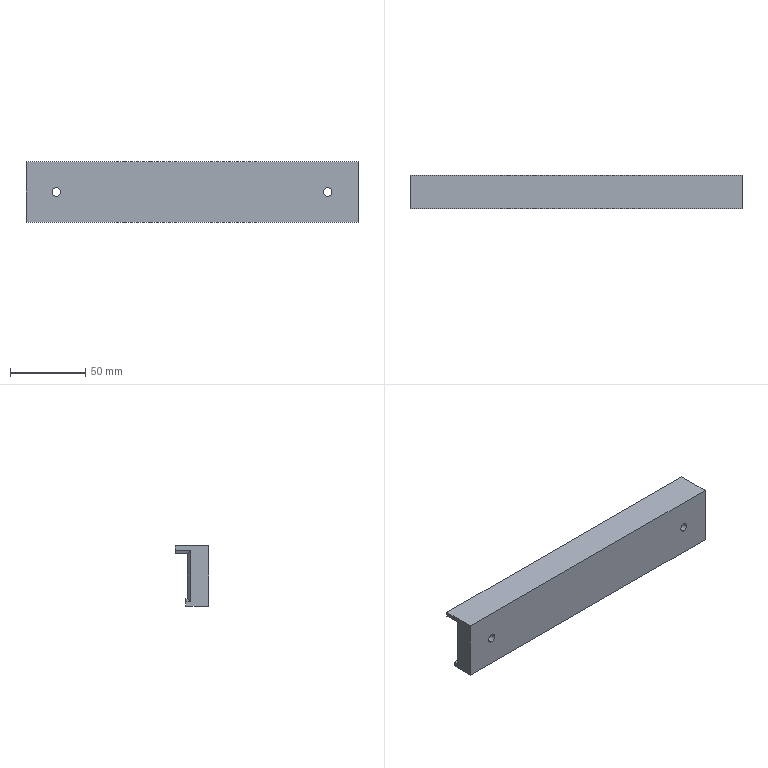Part | STEP file | (PA01.001.LX004) Belt Track | 1 solid | 26 faces | box 220 x 22 x 40 mm | volume 130807 mm3 | plane 18 | cylinder 8 | commonest cylinder face diameters 5.5 x4 10 x4